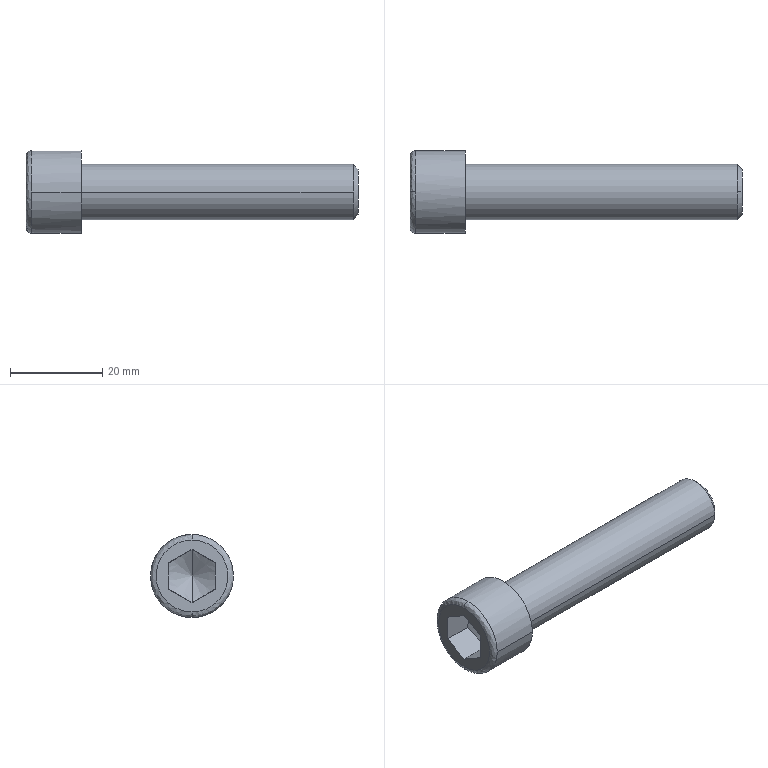Part | STEP file | DIN 912 - replaced by DIN EN ISO 4762 M12 x 60 | 1 solid | 21 faces | box 72 x 18 x 18 mm | volume 9169 mm3 | plane 9 | spline 4 | cylinder 4 | cone 4 | commonest cylinder face diameters 12 x2 18 x2